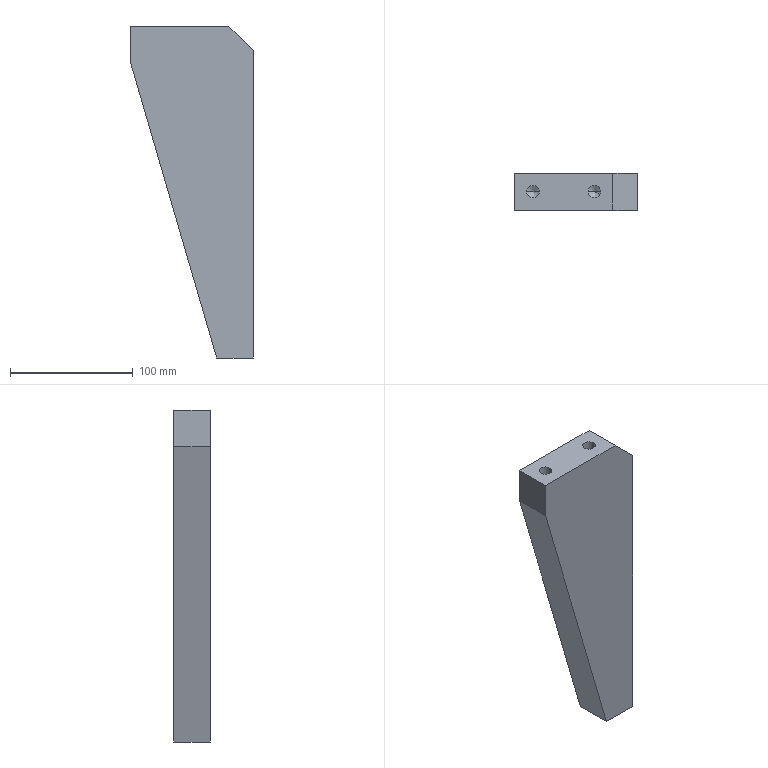Part | SolidWorks | features HoleWzd 2, Extrusion 1 | 1 solid | 32 faces | box 100 x 30 x 270 mm | volume 537159 mm3 | cylinder 12 | cone 12 | plane 8 | commonest cylinder face diameters 10.2 x12
STEP:
#1=CARTESIAN_POINT('',(-40.1,15.,240.75));
#2=VERTEX_POINT('',#1);
#3=CARTESIAN_POINT('',(-29.9,15.,240.75));
#4=VERTEX_POINT('',#3);
#5=CARTESIAN_POINT('',(-35.,15.,240.75));
#6=DIRECTION('',(0.,0.,1.));
#7=DIRECTION('',(1.,0.,0.));
#8=AXIS2_PLACEMENT_3D('',#5,#6,#7);
#9=CIRCLE('',#8,5.1);
#10=EDGE_CURVE('',#2,#4,#9,.T.);
#11=ORIENTED_EDGE('',*,*,#10,.F.);
#12=CARTESIAN_POINT('',(-40.1,15.,270.));
#13=VERTEX_POINT('',#12);
#14=CARTESIAN_POINT('',(-40.1,15.,270.));
#15=DIRECTION('',(0.,0.,1.));
#16=VECTOR('',#15,1000.);
#17=LINE('',#14,#16);
#18=EDGE_CURVE('',#2,#13,#17,.T.);
#19=ORIENTED_EDGE('',*,*,#18,.T.);
#20=CARTESIAN_POINT('',(-29.9,15.,270.));
#21=VERTEX_POINT('',#20);
#22=CARTESIAN_POINT('',(-35.,15.,270.));
#23=DIRECTION('',(0.,0.,1.));
#24=DIRECTION('',(1.,0.,0.));
#25=AXIS2_PLACEMENT_3D('',#22,#23,#24);
#26=CIRCLE('',#25,5.1);
#27=EDGE_CURVE('',#13,#21,#26,.T.);
#28=ORIENTED_EDGE('',*,*,#27,.T.);
#29=CARTESIAN_POINT('',(-29.9,15.,270.));
#30=DIRECTION('',(0.,0.,1.));
#31=VECTOR('',#30,1000.);
#32=LINE('',#29,#31);
#33=EDGE_CURVE('',#4,#21,#32,.T.);
#34=ORIENTED_EDGE('',*,*,#33,.F.);
#35=EDGE_LOOP('',(#11,#19,#28,#34));
#36=FACE_OUTER_BOUND('',#35,.T.);
#37=CARTESIAN_POINT('',(-35.,15.,270.));
#38=DIRECTION('',(0.,0.,1.));
#39=DIRECTION('',(1.,0.,0.));
#40=AXIS2_PLACEMENT_3D('',#37,#38,#39);
#41=CYLINDRICAL_SURFACE('',#40,5.1);
#42=ADVANCED_FACE('',(#36),#41,.F.);
#43=CARTESIAN_POINT('',(-35.,15.,237.686));
#44=VERTEX_POINT('',#43);
#45=CARTESIAN_POINT('',(-29.9,15.,240.75));
#46=DIRECTION('',(0.8572,0.,0.515));
#47=VECTOR('',#46,1000.);
#48=LINE('',#45,#47);
#49=EDGE_CURVE('',#44,#4,#48,.T.);
#50=ORIENTED_EDGE('',*,*,#49,.F.);
#51=CARTESIAN_POINT('',(-40.1,15.,240.75));
#52=DIRECTION('',(-0.8572,0.,0.515));
#53=VECTOR('',#52,1000.);
#54=LINE('',#51,#53);
#55=EDGE_CURVE('',#44,#2,#54,.T.);
#56=ORIENTED_EDGE('',*,*,#55,.T.);
#57=ORIENTED_EDGE('',*,*,#10,.T.);
#58=EDGE_LOOP('',(#50,#56,#57));
#59=FACE_OUTER_BOUND('',#58,.T.);
#60=CARTESIAN_POINT('',(-35.,15.,240.75));
#61=DIRECTION('',(0.,0.,1.));
#62=DIRECTION('',(1.,0.,0.));
#63=AXIS2_PLACEMENT_3D('',#60,#61,#62);
#64=CONICAL_SURFACE('',#63,5.1,1.03);
#65=ADVANCED_FACE('',(#59),#64,.F.);
#66=CARTESIAN_POINT('',(-90.1,15.,240.75));
#67=VERTEX_POINT('',#66);
#68=CARTESIAN_POINT('',(-79.9,15.,240.75));
#69=VERTEX_POINT('',#68);
#70=CARTESIAN_POINT('',(-85.,15.,240.75));
#71=DIRECTION('',(0.,0.,1.));
#72=DIRECTION('',(1.,0.,0.));
#73=AXIS2_PLACEMENT_3D('',#70,#71,#72);
#74=CIRCLE('',#73,5.1);
#75=EDGE_CURVE('',#67,#69,#74,.T.);
#76=ORIENTED_EDGE('',*,*,#75,.F.);
#77=CARTESIAN_POINT('',(-90.1,15.,270.));
#78=VERTEX_POINT('',#77);
#79=CARTESIAN_POINT('',(-90.1,15.,270.));
#80=DIRECTION('',(0.,0.,1.));
#81=VECTOR('',#80,1000.);
#82=LINE('',#79,#81);
#83=EDGE_CURVE('',#67,#78,#82,.T.);
#84=ORIENTED_EDGE('',*,*,#83,.T.);
#85=CARTESIAN_POINT('',(-79.9,15.,270.));
#86=VERTEX_POINT('',#85);
#87=CARTESIAN_POINT('',(-85.,15.,270.));
#88=DIRECTION('',(0.,0.,1.));
#89=DIRECTION('',(1.,0.,0.));
#90=AXIS2_PLACEMENT_3D('',#87,#88,#89);
#91=CIRCLE('',#90,5.1);
#92=EDGE_CURVE('',#78,#86,#91,.T.);
#93=ORIENTED_EDGE('',*,*,#92,.T.);
#94=CARTESIAN_POINT('',(-79.9,15.,270.));
#95=DIRECTION('',(0.,0.,1.));
#96=VECTOR('',#95,1000.);
#97=LINE('',#94,#96);
#98=EDGE_CURVE('',#69,#86,#97,.T.);
#99=ORIENTED_EDGE('',*,*,#98,.F.);
#100=EDGE_LOOP('',(#76,#84,#93,#99));
#101=FACE_OUTER_BOUND('',#100,.T.);
#102=CARTESIAN_POINT('',(-85.,15.,270.));
#103=DIRECTION('',(0.,0.,1.));
#104=DIRECTION('',(1.,0.,0.));
#105=AXIS2_PLACEMENT_3D('',#102,#103,#104);
#106=CYLINDRICAL_SURFACE('',#105,5.1);
#107=ADVANCED_FACE('',(#101),#106,.F.);
#108=CARTESIAN_POINT('',(-85.,15.,237.686));
#109=VERTEX_POINT('',#108);
#110=CARTESIAN_POINT('',(-79.9,15.,240.75));
#111=DIRECTION('',(0.8572,0.,0.515));
#112=VECTOR('',#111,1000.);
#113=LINE('',#110,#112);
#114=EDGE_CURVE('',#109,#69,#113,.T.);
#115=ORIENTED_EDGE('',*,*,#114,.F.);
#116=CARTESIAN_POINT('',(-90.1,15.,240.75));
#117=DIRECTION('',(-0.8572,0.,0.515));
#118=VECTOR('',#117,1000.);
#119=LINE('',#116,#118);
#120=EDGE_CURVE('',#109,#67,#119,.T.);
#121=ORIENTED_EDGE('',*,*,#120,.T.);
#122=ORIENTED_EDGE('',*,*,#75,.T.);
#123=EDGE_LOOP('',(#115,#121,#122));
#124=FACE_OUTER_BOUND('',#123,.T.);
#125=CARTESIAN_POINT('',(-85.,15.,240.75));
#126=DIRECTION('',(0.,0.,1.));
#127=DIRECTION('',(1.,0.,0.));
#128=AXIS2_PLACEMENT_3D('',#125,#126,#127);
#129=CONICAL_SURFACE('',#128,5.1,1.03);
#130=ADVANCED_FACE('',(#124),#129,.F.);
#131=CARTESIAN_POINT('',(-29.25,15.,240.1));
#132=VERTEX_POINT('',#131);
#133=CARTESIAN_POINT('',(-29.25,15.,229.9));
#134=VERTEX_POINT('',#133);
#135=CARTESIAN_POINT('',(-29.25,15.,235.));
#136=DIRECTION('',(1.,0.,0.));
#137=DIRECTION('',(0.,0.,-1.));
#138=AXIS2_PLACEMENT_3D('',#135,#136,#137);
#139=CIRCLE('',#138,5.1);
#140=EDGE_CURVE('',#132,#134,#139,.T.);
#141=ORIENTED_EDGE('',*,*,#140,.F.);
#142=CARTESIAN_POINT('',(0.,15.,240.1));
#143=VERTEX_POINT('',#142);
#144=CARTESIAN_POINT('',(0.,15.,240.1));
#145=DIRECTION('',(1.,0.,0.));
#146=VECTOR('',#145,1000.);
#147=LINE('',#144,#146);
#148=EDGE_CURVE('',#132,#143,#147,.T.);
#149=ORIENTED_EDGE('',*,*,#148,.T.);
#150=CARTESIAN_POINT('',(0.,15.,229.9));
#151=VERTEX_POINT('',#150);
#152=CARTESIAN_POINT('',(0.,15.,235.));
#153=DIRECTION('',(1.,0.,0.));
#154=DIRECTION('',(0.,0.,-1.));
#155=AXIS2_PLACEMENT_3D('',#152,#153,#154);
#156=CIRCLE('',#155,5.1);
#157=EDGE_CURVE('',#143,#151,#156,.T.);
#158=ORIENTED_EDGE('',*,*,#157,.T.);
#159=CARTESIAN_POINT('',(0.,15.,229.9));
#160=DIRECTION('',(1.,0.,0.));
#161=VECTOR('',#160,1000.);
#162=LINE('',#159,#161);
#163=EDGE_CURVE('',#134,#151,#162,.T.);
#164=ORIENTED_EDGE('',*,*,#163,.F.);
#165=EDGE_LOOP('',(#141,#149,#158,#164));
#166=FACE_OUTER_BOUND('',#165,.T.);
#167=CARTESIAN_POINT('',(0.,15.,235.));
#168=DIRECTION('',(1.,0.,0.));
#169=DIRECTION('',(0.,0.,-1.));
#170=AXIS2_PLACEMENT_3D('',#167,#168,#169);
#171=CYLINDRICAL_SURFACE('',#170,5.1);
#172=ADVANCED_FACE('',(#166),#171,.F.);
#173=CARTESIAN_POINT('',(-32.314,15.,235.));
#174=VERTEX_POINT('',#173);
#175=CARTESIAN_POINT('',(-29.25,15.,229.9));
#176=DIRECTION('',(0.515,0.,-0.8572));
#177=VECTOR('',#176,1000.);
#178=LINE('',#175,#177);
#179=EDGE_CURVE('',#174,#134,#178,.T.);
#180=ORIENTED_EDGE('',*,*,#179,.F.);
#181=CARTESIAN_POINT('',(-29.25,15.,240.1));
#182=DIRECTION('',(0.515,0.,0.8572));
#183=VECTOR('',#182,1000.);
#184=LINE('',#181,#183);
#185=EDGE_CURVE('',#174,#132,#184,.T.);
#186=ORIENTED_EDGE('',*,*,#185,.T.);
#187=ORIENTED_EDGE('',*,*,#140,.T.);
#188=EDGE_LOOP('',(#180,#186,#187));
#189=FACE_OUTER_BOUND('',#188,.T.);
#190=CARTESIAN_POINT('',(-29.25,15.,235.));
#191=DIRECTION('',(1.,0.,0.));
#192=DIRECTION('',(0.,0.,-1.));
#193=AXIS2_PLACEMENT_3D('',#190,#191,#192);
#194=CONICAL_SURFACE('',#193,5.1,1.03);
#195=ADVANCED_FACE('',(#189),#194,.F.);
#196=CARTESIAN_POINT('',(-29.25,15.,20.1));
#197=VERTEX_POINT('',#196);
#198=CARTESIAN_POINT('',(-29.25,15.,9.9));
#199=VERTEX_POINT('',#198);
#200=CARTESIAN_POINT('',(-29.25,15.,15.));
#201=DIRECTION('',(1.,0.,0.));
#202=DIRECTION('',(0.,0.,-1.));
#203=AXIS2_PLACEMENT_3D('',#200,#201,#202);
#204=CIRCLE('',#203,5.1);
#205=EDGE_CURVE('',#197,#199,#204,.T.);
#206=ORIENTED_EDGE('',*,*,#205,.F.);
#207=CARTESIAN_POINT('',(0.,15.,20.1));
#208=VERTEX_POINT('',#207);
#209=CARTESIAN_POINT('',(0.,15.,20.1));
#210=DIRECTION('',(1.,0.,0.));
#211=VECTOR('',#210,1000.);
#212=LINE('',#209,#211);
#213=EDGE_CURVE('',#197,#208,#212,.T.);
#214=ORIENTED_EDGE('',*,*,#213,.T.);
#215=CARTESIAN_POINT('',(0.,15.,9.9));
#216=VERTEX_POINT('',#215);
#217=CARTESIAN_POINT('',(0.,15.,15.));
#218=DIRECTION('',(1.,0.,0.));
#219=DIRECTION('',(0.,0.,-1.));
#220=AXIS2_PLACEMENT_3D('',#217,#218,#219);
#221=CIRCLE('',#220,5.1);
#222=EDGE_CURVE('',#208,#216,#221,.T.);
#223=ORIENTED_EDGE('',*,*,#222,.T.);
#224=CARTESIAN_POINT('',(0.,15.,9.9));
#225=DIRECTION('',(1.,0.,0.));
#226=VECTOR('',#225,1000.);
#227=LINE('',#224,#226);
#228=EDGE_CURVE('',#199,#216,#227,.T.);
#229=ORIENTED_EDGE('',*,*,#228,.F.);
#230=EDGE_LOOP('',(#206,#214,#223,#229));
#231=FACE_OUTER_BOUND('',#230,.T.);
#232=CARTESIAN_POINT('',(0.,15.,15.));
#233=DIRECTION('',(1.,0.,0.));
#234=DIRECTION('',(0.,0.,-1.));
#235=AXIS2_PLACEMENT_3D('',#232,#233,#234);
#236=CYLINDRICAL_SURFACE('',#235,5.1);
#237=ADVANCED_FACE('',(#231),#236,.F.);
#238=CARTESIAN_POINT('',(-32.314,15.,15.));
#239=VERTEX_POINT('',#238);
#240=CARTESIAN_POINT('',(-29.25,15.,9.9));
#241=DIRECTION('',(0.515,0.,-0.8572));
#242=VECTOR('',#241,1000.);
#243=LINE('',#240,#242);
#244=EDGE_CURVE('',#239,#199,#243,.T.);
#245=ORIENTED_EDGE('',*,*,#244,.F.);
#246=CARTESIAN_POINT('',(-29.25,15.,20.1));
#247=DIRECTION('',(0.515,0.,0.8572));
#248=VECTOR('',#247,1000.);
#249=LINE('',#246,#248);
#250=EDGE_CURVE('',#239,#197,#249,.T.);
#251=ORIENTED_EDGE('',*,*,#250,.T.);
#252=ORIENTED_EDGE('',*,*,#205,.T.);
#253=EDGE_LOOP('',(#245,#251,#252));
#254=FACE_OUTER_BOUND('',#253,.T.);
#255=CARTESIAN_POINT('',(-29.25,15.,15.));
#256=DIRECTION('',(1.,0.,0.));
#257=DIRECTION('',(0.,0.,-1.));
#258=AXIS2_PLACEMENT_3D('',#255,#256,#257);
#259=CONICAL_SURFACE('',#258,5.1,1.03);
#260=ADVANCED_FACE('',(#254),#259,.F.);
#261=CARTESIAN_POINT('',(-29.25,15.,93.433));
#262=VERTEX_POINT('',#261);
#263=CARTESIAN_POINT('',(-29.25,15.,83.233));
#264=VERTEX_POINT('',#263);
#265=CARTESIAN_POINT('',(-29.25,15.,88.333));
#266=DIRECTION('',(1.,0.,0.));
#267=DIRECTION('',(0.,0.,-1.));
#268=AXIS2_PLACEMENT_3D('',#265,#266,#267);
#269=CIRCLE('',#268,5.1);
#270=EDGE_CURVE('',#262,#264,#269,.T.);
#271=ORIENTED_EDGE('',*,*,#270,.F.);
#272=CARTESIAN_POINT('',(0.,15.,93.433));
#273=VERTEX_POINT('',#272);
#274=CARTESIAN_POINT('',(0.,15.,93.433));
#275=DIRECTION('',(1.,0.,0.));
#276=VECTOR('',#275,1000.);
#277=LINE('',#274,#276);
#278=EDGE_CURVE('',#262,#273,#277,.T.);
#279=ORIENTED_EDGE('',*,*,#278,.T.);
#280=CARTESIAN_POINT('',(0.,15.,83.233));
#281=VERTEX_POINT('',#280);
#282=CARTESIAN_POINT('',(0.,15.,88.333));
#283=DIRECTION('',(1.,0.,0.));
#284=DIRECTION('',(0.,0.,-1.));
#285=AXIS2_PLACEMENT_3D('',#282,#283,#284);
#286=CIRCLE('',#285,5.1);
#287=EDGE_CURVE('',#273,#281,#286,.T.);
#288=ORIENTED_EDGE('',*,*,#287,.T.);
#289=CARTESIAN_POINT('',(0.,15.,83.233));
#290=DIRECTION('',(1.,0.,0.));
#291=VECTOR('',#290,1000.);
#292=LINE('',#289,#291);
#293=EDGE_CURVE('',#264,#281,#292,.T.);
#294=ORIENTED_EDGE('',*,*,#293,.F.);
#295=EDGE_LOOP('',(#271,#279,#288,#294));
#296=FACE_OUTER_BOUND('',#295,.T.);
#297=CARTESIAN_POINT('',(0.,15.,88.333));
#298=DIRECTION('',(1.,0.,0.));
#299=DIRECTION('',(0.,0.,-1.));
#300=AXIS2_PLACEMENT_3D('',#297,#298,#299);
#301=CYLINDRICAL_SURFACE('',#300,5.1);
#302=ADVANCED_FACE('',(#296),#301,.F.);
#303=CARTESIAN_POINT('',(-32.314,15.,88.333));
#304=VERTEX_POINT('',#303);
#305=CARTESIAN_POINT('',(-29.25,15.,83.233));
#306=DIRECTION('',(0.515,0.,-0.8572));
#307=VECTOR('',#306,1000.);
#308=LINE('',#305,#307);
#309=EDGE_CURVE('',#304,#264,#308,.T.);
#310=ORIENTED_EDGE('',*,*,#309,.F.);
#311=CARTESIAN_POINT('',(-29.25,15.,93.433));
#312=DIRECTION('',(0.515,0.,0.8572));
#313=VECTOR('',#312,1000.);
#314=LINE('',#311,#313);
#315=EDGE_CURVE('',#304,#262,#314,.T.);
#316=ORIENTED_EDGE('',*,*,#315,.T.);
#317=ORIENTED_EDGE('',*,*,#270,.T.);
#318=EDGE_LOOP('',(#310,#316,#317));
#319=FACE_OUTER_BOUND('',#318,.T.);
#320=CARTESIAN_POINT('',(-29.25,15.,88.333));
#321=DIRECTION('',(1.,0.,0.));
#322=DIRECTION('',(0.,0.,-1.));
#323=AXIS2_PLACEMENT_3D('',#320,#321,#322);
#324=CONICAL_SURFACE('',#323,5.1,1.03);
#325=ADVANCED_FACE('',(#319),#324,.F.);
#326=CARTESIAN_POINT('',(-29.25,15.,166.767));
#327=VERTEX_POINT('',#326);
#328=CARTESIAN_POINT('',(-29.25,15.,156.567));
#329=VERTEX_POINT('',#328);
#330=CARTESIAN_POINT('',(-29.25,15.,161.667));
#331=DIRECTION('',(1.,0.,0.));
#332=DIRECTION('',(0.,0.,-1.));
#333=AXIS2_PLACEMENT_3D('',#330,#331,#332);
#334=CIRCLE('',#333,5.1);
#335=EDGE_CURVE('',#327,#329,#334,.T.);
#336=ORIENTED_EDGE('',*,*,#335,.F.);
#337=CARTESIAN_POINT('',(0.,15.,166.767));
#338=VERTEX_POINT('',#337);
#339=CARTESIAN_POINT('',(0.,15.,166.767));
#340=DIRECTION('',(1.,0.,0.));
#341=VECTOR('',#340,1000.);
#342=LINE('',#339,#341);
#343=EDGE_CURVE('',#327,#338,#342,.T.);
#344=ORIENTED_EDGE('',*,*,#343,.T.);
#345=CARTESIAN_POINT('',(0.,15.,156.567));
#346=VERTEX_POINT('',#345);
#347=CARTESIAN_POINT('',(0.,15.,161.667));
#348=DIRECTION('',(1.,0.,0.));
#349=DIRECTION('',(0.,0.,-1.));
#350=AXIS2_PLACEMENT_3D('',#347,#348,#349);
#351=CIRCLE('',#350,5.1);
#352=EDGE_CURVE('',#338,#346,#351,.T.);
#353=ORIENTED_EDGE('',*,*,#352,.T.);
#354=CARTESIAN_POINT('',(0.,15.,156.567));
#355=DIRECTION('',(1.,0.,0.));
#356=VECTOR('',#355,1000.);
#357=LINE('',#354,#356);
#358=EDGE_CURVE('',#329,#346,#357,.T.);
#359=ORIENTED_EDGE('',*,*,#358,.F.);
#360=EDGE_LOOP('',(#336,#344,#353,#359));
#361=FACE_OUTER_BOUND('',#360,.T.);
#362=CARTESIAN_POINT('',(0.,15.,161.667));
#363=DIRECTION('',(1.,0.,0.));
#364=DIRECTION('',(0.,0.,-1.));
#365=AXIS2_PLACEMENT_3D('',#362,#363,#364);
#366=CYLINDRICAL_SURFACE('',#365,5.1);
#367=ADVANCED_FACE('',(#361),#366,.F.);
#368=CARTESIAN_POINT('',(-32.314,15.,161.667));
#369=VERTEX_POINT('',#368);
#370=CARTESIAN_POINT('',(-29.25,15.,156.567));
#371=DIRECTION('',(0.515,0.,-0.8572));
#372=VECTOR('',#371,1000.);
#373=LINE('',#370,#372);
#374=EDGE_CURVE('',#369,#329,#373,.T.);
#375=ORIENTED_EDGE('',*,*,#374,.F.);
#376=CARTESIAN_POINT('',(-29.25,15.,166.767));
#377=DIRECTION('',(0.515,0.,0.8572));
#378=VECTOR('',#377,1000.);
#379=LINE('',#376,#378);
#380=EDGE_CURVE('',#369,#327,#379,.T.);
#381=ORIENTED_EDGE('',*,*,#380,.T.);
#382=ORIENTED_EDGE('',*,*,#335,.T.);
#383=EDGE_LOOP('',(#375,#381,#382));
#384=FACE_OUTER_BOUND('',#383,.T.);
#385=CARTESIAN_POINT('',(-29.25,15.,161.667));
#386=DIRECTION('',(1.,0.,0.));
#387=DIRECTION('',(0.,0.,-1.));
#388=AXIS2_PLACEMENT_3D('',#385,#386,#387);
#389=CONICAL_SURFACE('',#388,5.1,1.03);
#390=ADVANCED_FACE('',(#384),#389,.F.);
#391=CARTESIAN_POINT('',(0.,0.,0.));
#392=VERTEX_POINT('',#391);
#393=CARTESIAN_POINT('',(-30.,0.,0.));
#394=VERTEX_POINT('',#393);
#395=CARTESIAN_POINT('',(-30.,0.,0.));
#396=DIRECTION('',(-1.,0.,0.));
#397=VECTOR('',#396,1000.);
#398=LINE('',#395,#397);
#399=EDGE_CURVE('',#392,#394,#398,.T.);
#400=ORIENTED_EDGE('',*,*,#399,.T.);
#401=CARTESIAN_POINT('',(-30.,30.,0.));
#402=VERTEX_POINT('',#401);
#403=CARTESIAN_POINT('',(-30.,30.,0.));
#404=DIRECTION('',(0.,-1.,0.));
#405=VECTOR('',#404,1000.);
#406=LINE('',#403,#405);
#407=EDGE_CURVE('',#402,#394,#406,.T.);
#408=ORIENTED_EDGE('',*,*,#407,.F.);
#409=CARTESIAN_POINT('',(0.,30.,0.));
#410=VERTEX_POINT('',#409);
#411=CARTESIAN_POINT('',(-30.,30.,0.));
#412=DIRECTION('',(-1.,0.,0.));
#413=VECTOR('',#412,1000.);
#414=LINE('',#411,#413);
#415=EDGE_CURVE('',#410,#402,#414,.T.);
#416=ORIENTED_EDGE('',*,*,#415,.F.);
#417=CARTESIAN_POINT('',(0.,30.,0.));
#418=DIRECTION('',(0.,-1.,0.));
#419=VECTOR('',#418,1000.);
#420=LINE('',#417,#419);
#421=EDGE_CURVE('',#410,#392,#420,.T.);
#422=ORIENTED_EDGE('',*,*,#421,.T.);
#423=EDGE_LOOP('',(#400,#408,#416,#422));
#424=FACE_OUTER_BOUND('',#423,.T.);
#425=CARTESIAN_POINT('',(-30.,30.,0.));
#426=DIRECTION('',(0.,0.,1.));
#427=DIRECTION('',(1.,0.,0.));
#428=AXIS2_PLACEMENT_3D('',#425,#426,#427);
#429=PLANE('',#428);
#430=ADVANCED_FACE('',(#424),#429,.F.);
#431=CARTESIAN_POINT('',(-100.,0.,240.));
#432=VERTEX_POINT('',#431);
#433=CARTESIAN_POINT('',(-100.,0.,240.));
#434=DIRECTION('',(-0.28,0.,0.96));
#435=VECTOR('',#434,1000.);
#436=LINE('',#433,#435);
#437=EDGE_CURVE('',#394,#432,#436,.T.);
#438=ORIENTED_EDGE('',*,*,#437,.T.);
#439=CARTESIAN_POINT('',(-100.,30.,240.));
#440=VERTEX_POINT('',#439);
#441=CARTESIAN_POINT('',(-100.,30.,240.));
#442=DIRECTION('',(0.,-1.,0.));
#443=VECTOR('',#442,1000.);
#444=LINE('',#441,#443);
#445=EDGE_CURVE('',#440,#432,#444,.T.);
#446=ORIENTED_EDGE('',*,*,#445,.F.);
#447=CARTESIAN_POINT('',(-100.,30.,240.));
#448=DIRECTION('',(-0.28,0.,0.96));
#449=VECTOR('',#448,1000.);
#450=LINE('',#447,#449);
#451=EDGE_CURVE('',#402,#440,#450,.T.);
#452=ORIENTED_EDGE('',*,*,#451,.F.);
#453=ORIENTED_EDGE('',*,*,#407,.T.);
#454=EDGE_LOOP('',(#438,#446,#452,#453));
#455=FACE_OUTER_BOUND('',#454,.T.);
#456=CARTESIAN_POINT('',(-100.,30.,240.));
#457=DIRECTION('',(0.96,0.,0.28));
#458=DIRECTION('',(0.28,0.,-0.96));
#459=AXIS2_PLACEMENT_3D('',#456,#457,#458);
#460=PLANE('',#459);
#461=ADVANCED_FACE('',(#455),#460,.F.);
#462=CARTESIAN_POINT('',(-100.,0.,270.));
#463=VERTEX_POINT('',#462);
#464=CARTESIAN_POINT('',(-100.,0.,270.));
#465=DIRECTION('',(0.,0.,1.));
#466=VECTOR('',#465,1000.);
#467=LINE('',#464,#466);
#468=EDGE_CURVE('',#432,#463,#467,.T.);
#469=ORIENTED_EDGE('',*,*,#468,.T.);
#470=CARTESIAN_POINT('',(-100.,30.,270.));
#471=VERTEX_POINT('',#470);
#472=CARTESIAN_POINT('',(-100.,30.,270.));
#473=DIRECTION('',(0.,-1.,0.));
#474=VECTOR('',#473,1000.);
#475=LINE('',#472,#474);
#476=EDGE_CURVE('',#471,#463,#475,.T.);
#477=ORIENTED_EDGE('',*,*,#476,.F.);
#478=CARTESIAN_POINT('',(-100.,30.,270.));
#479=DIRECTION('',(0.,0.,1.));
#480=VECTOR('',#479,1000.);
#481=LINE('',#478,#480);
#482=EDGE_CURVE('',#440,#471,#481,.T.);
#483=ORIENTED_EDGE('',*,*,#482,.F.);
#484=ORIENTED_EDGE('',*,*,#445,.T.);
#485=EDGE_LOOP('',(#469,#477,#483,#484));
#486=FACE_OUTER_BOUND('',#485,.T.);
#487=CARTESIAN_POINT('',(-100.,30.,270.));
#488=DIRECTION('',(1.,0.,0.));
#489=DIRECTION('',(0.,0.,-1.));
#490=AXIS2_PLACEMENT_3D('',#487,#488,#489);
#491=PLANE('',#490);
#492=ADVANCED_FACE('',(#486),#491,.F.);
#493=CARTESIAN_POINT('',(-35.,15.,270.));
#494=DIRECTION('',(0.,0.,1.));
#495=DIRECTION('',(1.,0.,0.));
#496=AXIS2_PLACEMENT_3D('',#493,#494,#495);
#497=CIRCLE('',#496,5.1);
#498=EDGE_CURVE('',#21,#13,#497,.T.);
#499=ORIENTED_EDGE('',*,*,#498,.F.);
#500=ORIENTED_EDGE('',*,*,#27,.F.);
#501=EDGE_LOOP('',(#499,#500));
#502=FACE_BOUND('',#501,.T.);
#503=CARTESIAN_POINT('',(-85.,15.,270.));
#504=DIRECTION('',(0.,0.,1.));
#505=DIRECTION('',(1.,0.,0.));
#506=AXIS2_PLACEMENT_3D('',#503,#504,#505);
#507=CIRCLE('',#506,5.1);
#508=EDGE_CURVE('',#86,#78,#507,.T.);
#509=ORIENTED_EDGE('',*,*,#508,.F.);
#510=ORIENTED_EDGE('',*,*,#92,.F.);
#511=EDGE_LOOP('',(#509,#510));
#512=FACE_BOUND('',#511,.T.);
#513=CARTESIAN_POINT('',(-20.,0.,270.));
#514=VERTEX_POINT('',#513);
#515=CARTESIAN_POINT('',(-20.,0.,270.));
#516=DIRECTION('',(1.,0.,0.));
#517=VECTOR('',#516,1000.);
#518=LINE('',#515,#517);
#519=EDGE_CURVE('',#463,#514,#518,.T.);
#520=ORIENTED_EDGE('',*,*,#519,.T.);
#521=CARTESIAN_POINT('',(-20.,30.,270.));
#522=VERTEX_POINT('',#521);
#523=CARTESIAN_POINT('',(-20.,30.,270.));
#524=DIRECTION('',(0.,-1.,0.));
#525=VECTOR('',#524,1000.);
#526=LINE('',#523,#525);
#527=EDGE_CURVE('',#522,#514,#526,.T.);
#528=ORIENTED_EDGE('',*,*,#527,.F.);
#529=CARTESIAN_POINT('',(-20.,30.,270.));
#530=DIRECTION('',(1.,0.,0.));
#531=VECTOR('',#530,1000.);
#532=LINE('',#529,#531);
#533=EDGE_CURVE('',#471,#522,#532,.T.);
#534=ORIENTED_EDGE('',*,*,#533,.F.);
#535=ORIENTED_EDGE('',*,*,#476,.T.);
#536=EDGE_LOOP('',(#520,#528,#534,#535));
#537=FACE_OUTER_BOUND('',#536,.T.);
#538=CARTESIAN_POINT('',(-20.,30.,270.));
#539=DIRECTION('',(0.,0.,-1.));
#540=DIRECTION('',(-1.,0.,0.));
#541=AXIS2_PLACEMENT_3D('',#538,#539,#540);
#542=PLANE('',#541);
#543=ADVANCED_FACE('',(#502,#512,#537),#542,.F.);
#544=CARTESIAN_POINT('',(0.,0.,250.));
#545=VERTEX_POINT('',#544);
#546=CARTESIAN_POINT('',(0.,0.,250.));
#547=DIRECTION('',(0.7071,0.,-0.7071));
#548=VECTOR('',#547,1000.);
#549=LINE('',#546,#548);
#550=EDGE_CURVE('',#514,#545,#549,.T.);
#551=ORIENTED_EDGE('',*,*,#550,.T.);
#552=CARTESIAN_POINT('',(0.,30.,250.));
#553=VERTEX_POINT('',#552);
#554=CARTESIAN_POINT('',(0.,30.,250.));
#555=DIRECTION('',(0.,-1.,0.));
#556=VECTOR('',#555,1000.);
#557=LINE('',#554,#556);
#558=EDGE_CURVE('',#553,#545,#557,.T.);
#559=ORIENTED_EDGE('',*,*,#558,.F.);
#560=CARTESIAN_POINT('',(0.,30.,250.));
#561=DIRECTION('',(0.7071,0.,-0.7071));
#562=VECTOR('',#561,1000.);
#563=LINE('',#560,#562);
#564=EDGE_CURVE('',#522,#553,#563,.T.);
#565=ORIENTED_EDGE('',*,*,#564,.F.);
#566=ORIENTED_EDGE('',*,*,#527,.T.);
#567=EDGE_LOOP('',(#551,#559,#565,#566));
#568=FACE_OUTER_BOUND('',#567,.T.);
#569=CARTESIAN_POINT('',(0.,30.,250.));
#570=DIRECTION('',(-0.7071,0.,-0.7071));
#571=DIRECTION('',(-0.7071,0.,0.7071));
#572=AXIS2_PLACEMENT_3D('',#569,#570,#571);
#573=PLANE('',#572);
#574=ADVANCED_FACE('',(#568),#573,.F.);
#575=CARTESIAN_POINT('',(0.,15.,235.));
#576=DIRECTION('',(1.,0.,0.));
#577=DIRECTION('',(0.,0.,-1.));
#578=AXIS2_PLACEMENT_3D('',#575,#576,#577);
#579=CIRCLE('',#578,5.1);
#580=EDGE_CURVE('',#151,#143,#579,.T.);
#581=ORIENTED_EDGE('',*,*,#580,.F.);
#582=ORIENTED_EDGE('',*,*,#157,.F.);
#583=EDGE_LOOP('',(#581,#582));
#584=FACE_BOUND('',#583,.T.);
#585=CARTESIAN_POINT('',(0.,15.,15.));
#586=DIRECTION('',(1.,0.,0.));
#587=DIRECTION('',(0.,0.,-1.));
#588=AXIS2_PLACEMENT_3D('',#585,#586,#587);
#589=CIRCLE('',#588,5.1);
#590=EDGE_CURVE('',#216,#208,#589,.T.);
#591=ORIENTED_EDGE('',*,*,#590,.F.);
#592=ORIENTED_EDGE('',*,*,#222,.F.);
#593=EDGE_LOOP('',(#591,#592));
#594=FACE_BOUND('',#593,.T.);
#595=CARTESIAN_POINT('',(0.,15.,88.333));
#596=DIRECTION('',(1.,0.,0.));
#597=DIRECTION('',(0.,0.,-1.));
#598=AXIS2_PLACEMENT_3D('',#595,#596,#597);
#599=CIRCLE('',#598,5.1);
#600=EDGE_CURVE('',#281,#273,#599,.T.);
#601=ORIENTED_EDGE('',*,*,#600,.F.);
#602=ORIENTED_EDGE('',*,*,#287,.F.);
#603=EDGE_LOOP('',(#601,#602));
#604=FACE_BOUND('',#603,.T.);
#605=CARTESIAN_POINT('',(0.,15.,161.667));
#606=DIRECTION('',(1.,0.,0.));
#607=DIRECTION('',(0.,0.,-1.));
#608=AXIS2_PLACEMENT_3D('',#605,#606,#607);
#609=CIRCLE('',#608,5.1);
#610=EDGE_CURVE('',#346,#338,#609,.T.);
#611=ORIENTED_EDGE('',*,*,#610,.F.);
#612=ORIENTED_EDGE('',*,*,#352,.F.);
#613=EDGE_LOOP('',(#611,#612));
#614=FACE_BOUND('',#613,.T.);
#615=CARTESIAN_POINT('',(0.,0.,0.));
#616=DIRECTION('',(0.,0.,-1.));
#617=VECTOR('',#616,1000.);
#618=LINE('',#615,#617);
#619=EDGE_CURVE('',#545,#392,#618,.T.);
#620=ORIENTED_EDGE('',*,*,#619,.T.);
#621=ORIENTED_EDGE('',*,*,#421,.F.);
#622=CARTESIAN_POINT('',(0.,30.,0.));
#623=DIRECTION('',(0.,0.,-1.));
#624=VECTOR('',#623,1000.);
#625=LINE('',#622,#624);
#626=EDGE_CURVE('',#553,#410,#625,.T.);
#627=ORIENTED_EDGE('',*,*,#626,.F.);
#628=ORIENTED_EDGE('',*,*,#558,.T.);
#629=EDGE_LOOP('',(#620,#621,#627,#628));
#630=FACE_OUTER_BOUND('',#629,.T.);
#631=CARTESIAN_POINT('',(0.,30.,0.));
#632=DIRECTION('',(-1.,0.,0.));
#633=DIRECTION('',(0.,0.,1.));
#634=AXIS2_PLACEMENT_3D('',#631,#632,#633);
#635=PLANE('',#634);
#636=ADVANCED_FACE('',(#584,#594,#604,#614,#630),#635,.F.);
#637=ORIENTED_EDGE('',*,*,#415,.T.);
#638=ORIENTED_EDGE('',*,*,#451,.T.);
#639=ORIENTED_EDGE('',*,*,#482,.T.);
#640=ORIENTED_EDGE('',*,*,#533,.T.);
#641=ORIENTED_EDGE('',*,*,#564,.T.);
#642=ORIENTED_EDGE('',*,*,#626,.T.);
#643=EDGE_LOOP('',(#637,#638,#639,#640,#641,#642));
#644=FACE_OUTER_BOUND('',#643,.T.);
#645=CARTESIAN_POINT('',(0.,30.,0.));
#646=DIRECTION('',(0.,-1.,0.));
#647=DIRECTION('',(0.,0.,-1.));
#648=AXIS2_PLACEMENT_3D('',#645,#646,#647);
#649=PLANE('',#648);
#650=ADVANCED_FACE('',(#644),#649,.F.);
#651=ORIENTED_EDGE('',*,*,#399,.F.);
#652=ORIENTED_EDGE('',*,*,#619,.F.);
#653=ORIENTED_EDGE('',*,*,#550,.F.);
#654=ORIENTED_EDGE('',*,*,#519,.F.);
#655=ORIENTED_EDGE('',*,*,#468,.F.);
#656=ORIENTED_EDGE('',*,*,#437,.F.);
#657=EDGE_LOOP('',(#651,#652,#653,#654,#655,#656));
#658=FACE_OUTER_BOUND('',#657,.T.);
#659=CARTESIAN_POINT('',(0.,0.,0.));
#660=DIRECTION('',(0.,-1.,0.));
#661=DIRECTION('',(0.,0.,-1.));
#662=AXIS2_PLACEMENT_3D('',#659,#660,#661);
#663=PLANE('',#662);
#664=ADVANCED_FACE('',(#658),#663,.T.);
#665=ORIENTED_EDGE('',*,*,#380,.F.);
#666=ORIENTED_EDGE('',*,*,#374,.T.);
#667=CARTESIAN_POINT('',(-29.25,15.,161.667));
#668=DIRECTION('',(1.,0.,0.));
#669=DIRECTION('',(0.,0.,-1.));
#670=AXIS2_PLACEMENT_3D('',#667,#668,#669);
#671=CIRCLE('',#670,5.1);
#672=EDGE_CURVE('',#329,#327,#671,.T.);
#673=ORIENTED_EDGE('',*,*,#672,.T.);
#674=EDGE_LOOP('',(#665,#666,#673));
#675=FACE_OUTER_BOUND('',#674,.T.);
#676=CARTESIAN_POINT('',(-29.25,15.,161.667));
#677=DIRECTION('',(1.,0.,0.));
#678=DIRECTION('',(0.,0.,-1.));
#679=AXIS2_PLACEMENT_3D('',#676,#677,#678);
#680=CONICAL_SURFACE('',#679,5.1,1.03);
#681=ADVANCED_FACE('',(#675),#680,.F.);
#682=ORIENTED_EDGE('',*,*,#343,.F.);
#683=ORIENTED_EDGE('',*,*,#672,.F.);
#684=ORIENTED_EDGE('',*,*,#358,.T.);
#685=ORIENTED_EDGE('',*,*,#610,.T.);
#686=EDGE_LOOP('',(#682,#683,#684,#685));
#687=FACE_OUTER_BOUND('',#686,.T.);
#688=CARTESIAN_POINT('',(0.,15.,161.667));
#689=DIRECTION('',(1.,0.,0.));
#690=DIRECTION('',(0.,0.,-1.));
#691=AXIS2_PLACEMENT_3D('',#688,#689,#690);
#692=CYLINDRICAL_SURFACE('',#691,5.1);
#693=ADVANCED_FACE('',(#687),#692,.F.);
#694=ORIENTED_EDGE('',*,*,#315,.F.);
#695=ORIENTED_EDGE('',*,*,#309,.T.);
#696=CARTESIAN_POINT('',(-29.25,15.,88.333));
#697=DIRECTION('',(1.,0.,0.));
#698=DIRECTION('',(0.,0.,-1.));
#699=AXIS2_PLACEMENT_3D('',#696,#697,#698);
#700=CIRCLE('',#699,5.1);
#701=EDGE_CURVE('',#264,#262,#700,.T.);
#702=ORIENTED_EDGE('',*,*,#701,.T.);
#703=EDGE_LOOP('',(#694,#695,#702));
#704=FACE_OUTER_BOUND('',#703,.T.);
#705=CARTESIAN_POINT('',(-29.25,15.,88.333));
#706=DIRECTION('',(1.,0.,0.));
#707=DIRECTION('',(0.,0.,-1.));
#708=AXIS2_PLACEMENT_3D('',#705,#706,#707);
#709=CONICAL_SURFACE('',#708,5.1,1.03);
#710=ADVANCED_FACE('',(#704),#709,.F.);
#711=ORIENTED_EDGE('',*,*,#278,.F.);
#712=ORIENTED_EDGE('',*,*,#701,.F.);
#713=ORIENTED_EDGE('',*,*,#293,.T.);
#714=ORIENTED_EDGE('',*,*,#600,.T.);
#715=EDGE_LOOP('',(#711,#712,#713,#714));
#716=FACE_OUTER_BOUND('',#715,.T.);
#717=CARTESIAN_POINT('',(0.,15.,88.333));
#718=DIRECTION('',(1.,0.,0.));
#719=DIRECTION('',(0.,0.,-1.));
#720=AXIS2_PLACEMENT_3D('',#717,#718,#719);
#721=CYLINDRICAL_SURFACE('',#720,5.1);
#722=ADVANCED_FACE('',(#716),#721,.F.);
#723=ORIENTED_EDGE('',*,*,#250,.F.);
#724=ORIENTED_EDGE('',*,*,#244,.T.);
#725=CARTESIAN_POINT('',(-29.25,15.,15.));
#726=DIRECTION('',(1.,0.,0.));
#727=DIRECTION('',(0.,0.,-1.));
#728=AXIS2_PLACEMENT_3D('',#725,#726,#727);
#729=CIRCLE('',#728,5.1);
#730=EDGE_CURVE('',#199,#197,#729,.T.);
#731=ORIENTED_EDGE('',*,*,#730,.T.);
#732=EDGE_LOOP('',(#723,#724,#731));
#733=FACE_OUTER_BOUND('',#732,.T.);
#734=CARTESIAN_POINT('',(-29.25,15.,15.));
#735=DIRECTION('',(1.,0.,0.));
#736=DIRECTION('',(0.,0.,-1.));
#737=AXIS2_PLACEMENT_3D('',#734,#735,#736);
#738=CONICAL_SURFACE('',#737,5.1,1.03);
#739=ADVANCED_FACE('',(#733),#738,.F.);
#740=ORIENTED_EDGE('',*,*,#213,.F.);
#741=ORIENTED_EDGE('',*,*,#730,.F.);
#742=ORIENTED_EDGE('',*,*,#228,.T.);
#743=ORIENTED_EDGE('',*,*,#590,.T.);
#744=EDGE_LOOP('',(#740,#741,#742,#743));
#745=FACE_OUTER_BOUND('',#744,.T.);
#746=CARTESIAN_POINT('',(0.,15.,15.));
#747=DIRECTION('',(1.,0.,0.));
#748=DIRECTION('',(0.,0.,-1.));
#749=AXIS2_PLACEMENT_3D('',#746,#747,#748);
#750=CYLINDRICAL_SURFACE('',#749,5.1);
#751=ADVANCED_FACE('',(#745),#750,.F.);
#752=ORIENTED_EDGE('',*,*,#185,.F.);
#753=ORIENTED_EDGE('',*,*,#179,.T.);
#754=CARTESIAN_POINT('',(-29.25,15.,235.));
#755=DIRECTION('',(1.,0.,0.));
#756=DIRECTION('',(0.,0.,-1.));
#757=AXIS2_PLACEMENT_3D('',#754,#755,#756);
#758=CIRCLE('',#757,5.1);
#759=EDGE_CURVE('',#134,#132,#758,.T.);
#760=ORIENTED_EDGE('',*,*,#759,.T.);
#761=EDGE_LOOP('',(#752,#753,#760));
#762=FACE_OUTER_BOUND('',#761,.T.);
#763=CARTESIAN_POINT('',(-29.25,15.,235.));
#764=DIRECTION('',(1.,0.,0.));
#765=DIRECTION('',(0.,0.,-1.));
#766=AXIS2_PLACEMENT_3D('',#763,#764,#765);
#767=CONICAL_SURFACE('',#766,5.1,1.03);
#768=ADVANCED_FACE('',(#762),#767,.F.);
#769=ORIENTED_EDGE('',*,*,#148,.F.);
#770=ORIENTED_EDGE('',*,*,#759,.F.);
#771=ORIENTED_EDGE('',*,*,#163,.T.);
#772=ORIENTED_EDGE('',*,*,#580,.T.);
#773=EDGE_LOOP('',(#769,#770,#771,#772));
#774=FACE_OUTER_BOUND('',#773,.T.);
#775=CARTESIAN_POINT('',(0.,15.,235.));
#776=DIRECTION('',(1.,0.,0.));
#777=DIRECTION('',(0.,0.,-1.));
#778=AXIS2_PLACEMENT_3D('',#775,#776,#777);
#779=CYLINDRICAL_SURFACE('',#778,5.1);
#780=ADVANCED_FACE('',(#774),#779,.F.);
#781=ORIENTED_EDGE('',*,*,#120,.F.);
#782=ORIENTED_EDGE('',*,*,#114,.T.);
#783=CARTESIAN_POINT('',(-85.,15.,240.75));
#784=DIRECTION('',(0.,0.,1.));
#785=DIRECTION('',(1.,0.,0.));
#786=AXIS2_PLACEMENT_3D('',#783,#784,#785);
#787=CIRCLE('',#786,5.1);
#788=EDGE_CURVE('',#69,#67,#787,.T.);
#789=ORIENTED_EDGE('',*,*,#788,.T.);
#790=EDGE_LOOP('',(#781,#782,#789));
#791=FACE_OUTER_BOUND('',#790,.T.);
#792=CARTESIAN_POINT('',(-85.,15.,240.75));
#793=DIRECTION('',(0.,0.,1.));
#794=DIRECTION('',(1.,0.,0.));
#795=AXIS2_PLACEMENT_3D('',#792,#793,#794);
#796=CONICAL_SURFACE('',#795,5.1,1.03);
#797=ADVANCED_FACE('',(#791),#796,.F.);
#798=ORIENTED_EDGE('',*,*,#83,.F.);
#799=ORIENTED_EDGE('',*,*,#788,.F.);
#800=ORIENTED_EDGE('',*,*,#98,.T.);
#801=ORIENTED_EDGE('',*,*,#508,.T.);
#802=EDGE_LOOP('',(#798,#799,#800,#801));
#803=FACE_OUTER_BOUND('',#802,.T.);
#804=CARTESIAN_POINT('',(-85.,15.,270.));
#805=DIRECTION('',(0.,0.,1.));
#806=DIRECTION('',(1.,0.,0.));
#807=AXIS2_PLACEMENT_3D('',#804,#805,#806);
#808=CYLINDRICAL_SURFACE('',#807,5.1);
#809=ADVANCED_FACE('',(#803),#808,.F.);
#810=ORIENTED_EDGE('',*,*,#55,.F.);
#811=ORIENTED_EDGE('',*,*,#49,.T.);
#812=CARTESIAN_POINT('',(-35.,15.,240.75));
#813=DIRECTION('',(0.,0.,1.));
#814=DIRECTION('',(1.,0.,0.));
#815=AXIS2_PLACEMENT_3D('',#812,#813,#814);
#816=CIRCLE('',#815,5.1);
#817=EDGE_CURVE('',#4,#2,#816,.T.);
#818=ORIENTED_EDGE('',*,*,#817,.T.);
#819=EDGE_LOOP('',(#810,#811,#818));
#820=FACE_OUTER_BOUND('',#819,.T.);
#821=CARTESIAN_POINT('',(-35.,15.,240.75));
#822=DIRECTION('',(0.,0.,1.));
#823=DIRECTION('',(1.,0.,0.));
#824=AXIS2_PLACEMENT_3D('',#821,#822,#823);
#825=CONICAL_SURFACE('',#824,5.1,1.03);
#826=ADVANCED_FACE('',(#820),#825,.F.);
#827=ORIENTED_EDGE('',*,*,#18,.F.);
#828=ORIENTED_EDGE('',*,*,#817,.F.);
#829=ORIENTED_EDGE('',*,*,#33,.T.);
#830=ORIENTED_EDGE('',*,*,#498,.T.);
#831=EDGE_LOOP('',(#827,#828,#829,#830));
#832=FACE_OUTER_BOUND('',#831,.T.);
#833=CARTESIAN_POINT('',(-35.,15.,270.));
#834=DIRECTION('',(0.,0.,1.));
#835=DIRECTION('',(1.,0.,0.));
#836=AXIS2_PLACEMENT_3D('',#833,#834,#835);
#837=CYLINDRICAL_SURFACE('',#836,5.1);
#838=ADVANCED_FACE('',(#832),#837,.F.);
#839=CLOSED_SHELL('',(#42,#65,#107,#130,#172,#195,#237,#260,#302,#325,#367,#390,#430,#461,#492,#543,#574,#636,#650,#664,#681,#693,#710,#722,#739,#751,#768,#780,#797,#809,#826,#838));
#840=MANIFOLD_SOLID_BREP('',#839);
#841=CARTESIAN_POINT('',(0.,0.,0.));
#842=DIRECTION('',(0.,0.,1.));
#843=DIRECTION('',(1.,0.,0.));
#844=AXIS2_PLACEMENT_3D('',#841,#842,#843);
#845=(LENGTH_UNIT()NAMED_UNIT(*)SI_UNIT(.MILLI.,.METRE.));
#846=UNCERTAINTY_MEASURE_WITH_UNIT(LENGTH_MEASURE(0.00001),#845,'','');
#847=(NAMED_UNIT(*)PLANE_ANGLE_UNIT()SI_UNIT($,.RADIAN.));
#848=(NAMED_UNIT(*)SI_UNIT($,.STERADIAN.)SOLID_ANGLE_UNIT());
#849=(GEOMETRIC_REPRESENTATION_CONTEXT(3)GLOBAL_UNCERTAINTY_ASSIGNED_CONTEXT((#846))GLOBAL_UNIT_ASSIGNED_CONTEXT((#845,#847,#848))REPRESENTATION_CONTEXT('',''));
#850=ADVANCED_BREP_SHAPE_REPRESENTATION('',(#840,#844),#849);